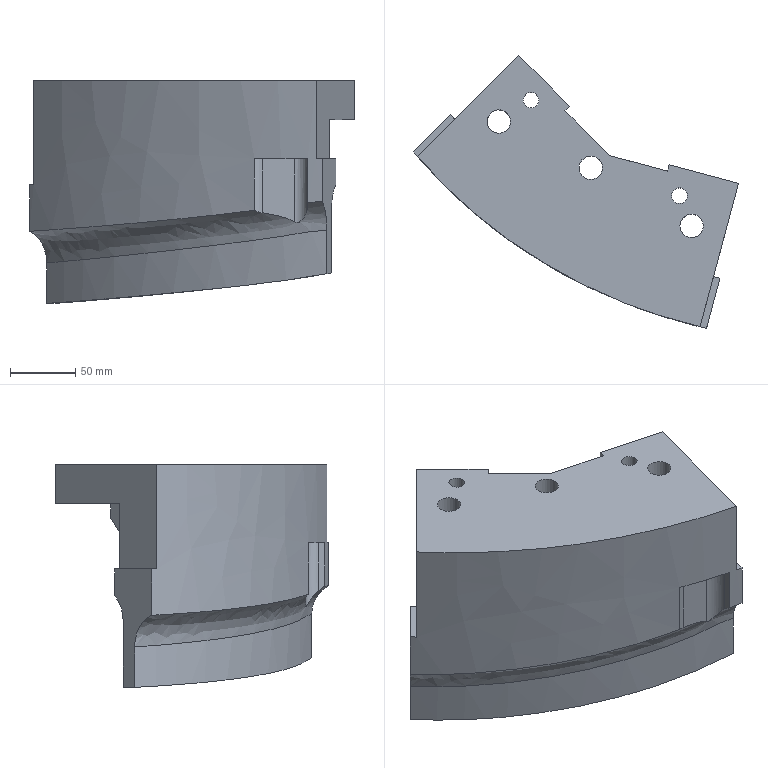Part | NX | features solid 2 | 1 solid | 48 faces | box 249.401 x 209.376 x 170.933 mm | volume 1735897 mm3 | plane 30 | cylinder 10 | spline 8 | commonest cylinder face diameters 18 x3 26 x3 12 x2 20 x2